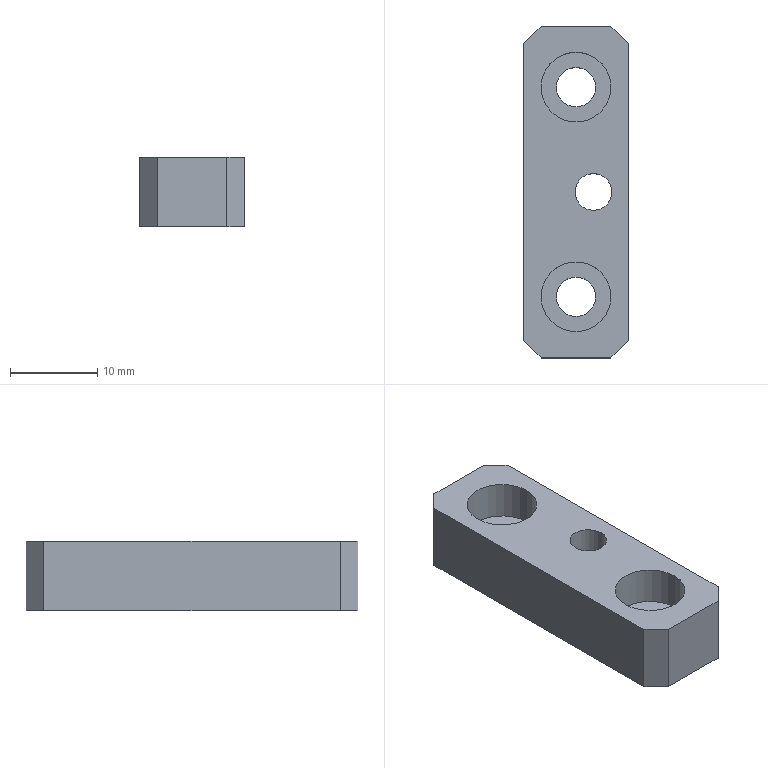Part | STEP file | (PA01.001.LX010) Clamp Block | 1 solid | 22 faces | box 12 x 38 x 8 mm | volume 2916 mm3 | plane 12 | cylinder 10 | commonest cylinder face diameters 4.5 x4 8 x4 4.2 x2